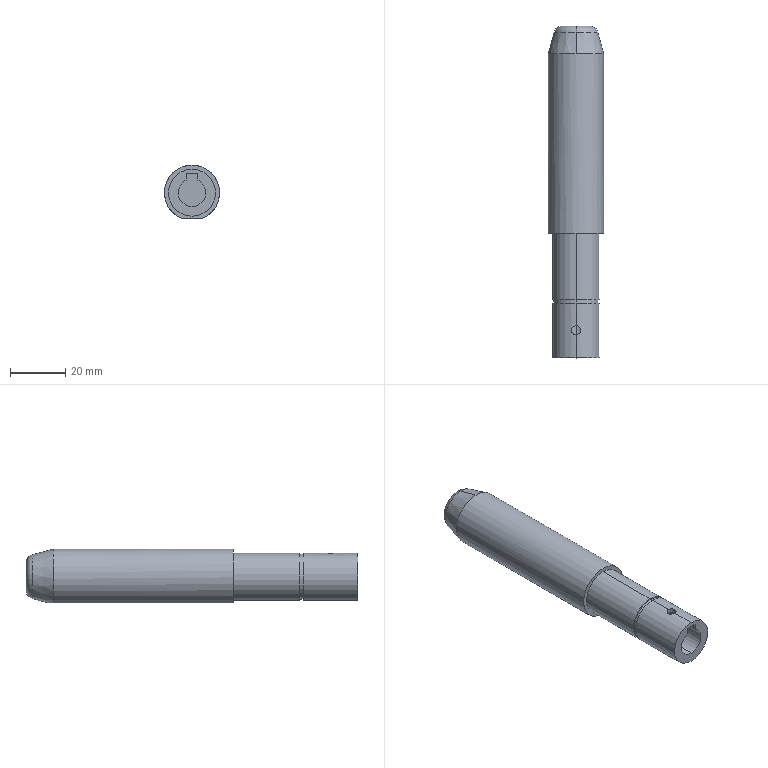Part | STEP file | QA-FC09 | 1 solid | 25 faces | box 20 x 120 x 19.5 mm | volume 30201 mm3 | cylinder 11 | plane 10 | torus 2 | cone 2 | commonest cylinder face diameters 17 x4 3.3 x2 10 x2 16.2 x2 20 x1